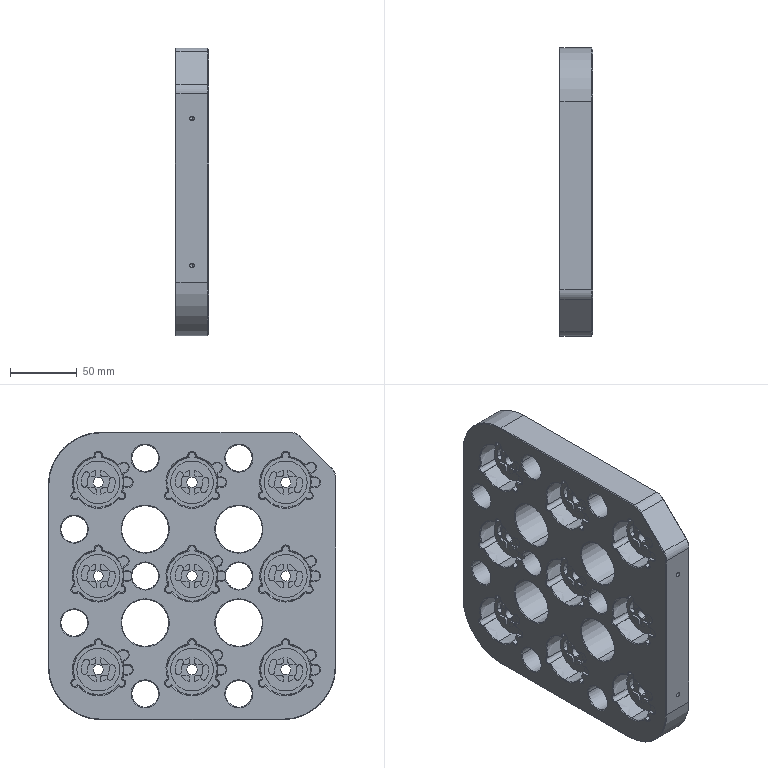Part | SolidWorks | features ICE 14, MoveCopyBody 7, MoveFace 6, Chamfer 4, LPattern 4, Cut 3, Fillet 3, Stock 2, Extrusion 1, HoleWzd 1 | 1 solid | 733 faces | box 25 x 215 x 215 mm | volume 796831 mm3 | cylinder 255 | plane 253 | cone 225 | commonest cylinder face diameters 4.5 x54 4 x36 18 x36 7 x20 7.55 x18 16.293 x18